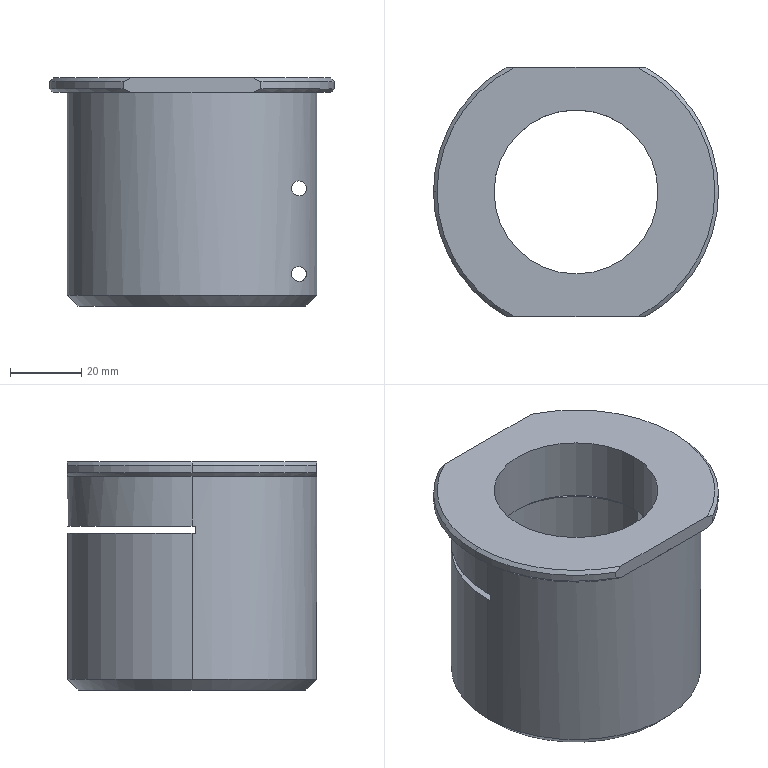Part | STEP file | QA-TE02 | 1 solid | 46 faces | box 80 x 70 x 64 mm | volume 121771 mm3 | cylinder 24 | plane 13 | cone 9 | commonest cylinder face diameters 10 x6 4.2 x4 5.5 x4 70 x3 80 x3 46 x2